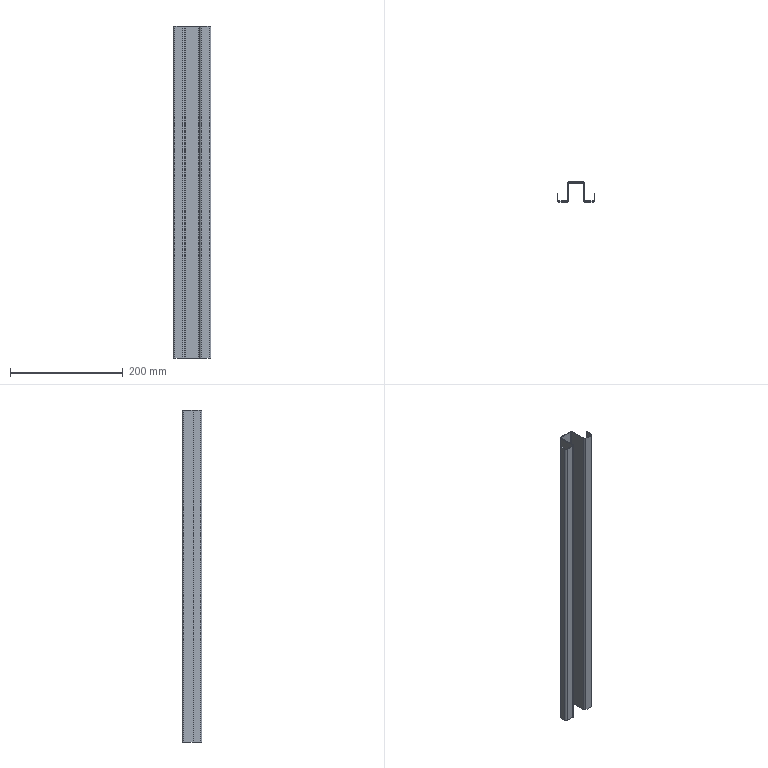Part | SolidWorks | features FlatPattern 1, SMBaseFlange 1, SheetMetal 1 | 1 solid | 54 faces | box 67 x 35 x 590 mm | volume 137357 mm3 | plane 42 | cylinder 12 | commonest cylinder face diameters 3 x6 6 x6
STEP:
#1=CARTESIAN_POINT('',(-17.662,-4.135,590.));
#2=VERTEX_POINT('',#1);
#3=CARTESIAN_POINT('',(-17.662,-5.635,590.));
#4=VERTEX_POINT('',#3);
#5=CARTESIAN_POINT('',(-17.662,-4.135,590.));
#6=DIRECTION('',(0.,-1.,0.));
#7=VECTOR('',#6,1000.);
#8=LINE('',#5,#7);
#9=EDGE_CURVE('',#2,#4,#8,.T.);
#10=ORIENTED_EDGE('',*,*,#9,.F.);
#11=CARTESIAN_POINT('',(-19.162,-2.635,590.));
#12=VERTEX_POINT('',#11);
#13=CARTESIAN_POINT('',(-17.662,-2.635,590.));
#14=DIRECTION('',(0.,0.,1.));
#15=DIRECTION('',(-1.,0.,0.));
#16=AXIS2_PLACEMENT_3D('',#13,#14,#15);
#17=CIRCLE('',#16,1.5);
#18=EDGE_CURVE('',#12,#2,#17,.T.);
#19=ORIENTED_EDGE('',*,*,#18,.F.);
#20=CARTESIAN_POINT('',(-20.662,-2.635,590.));
#21=VERTEX_POINT('',#20);
#22=CARTESIAN_POINT('',(-20.662,-2.635,590.));
#23=DIRECTION('',(1.,0.,0.));
#24=VECTOR('',#23,1000.);
#25=LINE('',#22,#24);
#26=EDGE_CURVE('',#21,#12,#25,.T.);
#27=ORIENTED_EDGE('',*,*,#26,.F.);
#28=CARTESIAN_POINT('',(-17.662,-2.635,590.));
#29=DIRECTION('',(0.,0.,1.));
#30=DIRECTION('',(1.,0.,0.));
#31=AXIS2_PLACEMENT_3D('',#28,#29,#30);
#32=CIRCLE('',#31,3.);
#33=EDGE_CURVE('',#21,#4,#32,.T.);
#34=ORIENTED_EDGE('',*,*,#33,.T.);
#35=EDGE_LOOP('',(#10,#19,#27,#34));
#36=FACE_OUTER_BOUND('',#35,.T.);
#37=CARTESIAN_POINT('',(-17.662,-4.135,590.));
#38=DIRECTION('',(0.,0.,1.));
#39=DIRECTION('',(1.,0.,0.));
#40=AXIS2_PLACEMENT_3D('',#37,#38,#39);
#41=PLANE('',#40);
#42=ADVANCED_FACE('',(#36),#41,.T.);
#43=CARTESIAN_POINT('',(-3.662,-4.135,590.));
#44=VERTEX_POINT('',#43);
#45=CARTESIAN_POINT('',(-19.162,-4.135,590.));
#46=DIRECTION('',(1.,0.,0.));
#47=VECTOR('',#46,1000.);
#48=LINE('',#45,#47);
#49=EDGE_CURVE('',#2,#44,#48,.T.);
#50=ORIENTED_EDGE('',*,*,#49,.F.);
#51=ORIENTED_EDGE('',*,*,#9,.T.);
#52=CARTESIAN_POINT('',(-3.662,-5.635,590.));
#53=VERTEX_POINT('',#52);
#54=CARTESIAN_POINT('',(-19.162,-5.635,590.));
#55=DIRECTION('',(1.,0.,0.));
#56=VECTOR('',#55,1000.);
#57=LINE('',#54,#56);
#58=EDGE_CURVE('',#4,#53,#57,.T.);
#59=ORIENTED_EDGE('',*,*,#58,.T.);
#60=CARTESIAN_POINT('',(-3.662,-5.635,590.));
#61=DIRECTION('',(0.,1.,0.));
#62=VECTOR('',#61,1000.);
#63=LINE('',#60,#62);
#64=EDGE_CURVE('',#53,#44,#63,.T.);
#65=ORIENTED_EDGE('',*,*,#64,.T.);
#66=EDGE_LOOP('',(#50,#51,#59,#65));
#67=FACE_OUTER_BOUND('',#66,.T.);
#68=CARTESIAN_POINT('',(-20.662,-2.635,590.));
#69=DIRECTION('',(0.,0.,1.));
#70=DIRECTION('',(1.,0.,0.));
#71=AXIS2_PLACEMENT_3D('',#68,#69,#70);
#72=PLANE('',#71);
#73=ADVANCED_FACE('',(#67),#72,.T.);
#74=CARTESIAN_POINT('',(-19.162,-2.635,0.));
#75=VERTEX_POINT('',#74);
#76=CARTESIAN_POINT('',(-20.662,-2.635,0.));
#77=VERTEX_POINT('',#76);
#78=CARTESIAN_POINT('',(-19.162,-2.635,0.));
#79=DIRECTION('',(-1.,0.,0.));
#80=VECTOR('',#79,1000.);
#81=LINE('',#78,#80);
#82=EDGE_CURVE('',#75,#77,#81,.T.);
#83=ORIENTED_EDGE('',*,*,#82,.F.);
#84=CARTESIAN_POINT('',(-17.662,-4.135,0.));
#85=VERTEX_POINT('',#84);
#86=CARTESIAN_POINT('',(-17.662,-2.635,0.));
#87=DIRECTION('',(0.,0.,1.));
#88=DIRECTION('',(-1.,0.,0.));
#89=AXIS2_PLACEMENT_3D('',#86,#87,#88);
#90=CIRCLE('',#89,1.5);
#91=EDGE_CURVE('',#75,#85,#90,.T.);
#92=ORIENTED_EDGE('',*,*,#91,.T.);
#93=CARTESIAN_POINT('',(-17.662,-5.635,0.));
#94=VERTEX_POINT('',#93);
#95=CARTESIAN_POINT('',(-17.662,-5.635,0.));
#96=DIRECTION('',(0.,1.,0.));
#97=VECTOR('',#96,1000.);
#98=LINE('',#95,#97);
#99=EDGE_CURVE('',#94,#85,#98,.T.);
#100=ORIENTED_EDGE('',*,*,#99,.F.);
#101=CARTESIAN_POINT('',(-17.662,-2.635,0.));
#102=DIRECTION('',(0.,0.,1.));
#103=DIRECTION('',(1.,0.,0.));
#104=AXIS2_PLACEMENT_3D('',#101,#102,#103);
#105=CIRCLE('',#104,3.);
#106=EDGE_CURVE('',#77,#94,#105,.T.);
#107=ORIENTED_EDGE('',*,*,#106,.F.);
#108=EDGE_LOOP('',(#83,#92,#100,#107));
#109=FACE_OUTER_BOUND('',#108,.T.);
#110=CARTESIAN_POINT('',(-19.162,-2.635,0.));
#111=DIRECTION('',(0.,0.,-1.));
#112=DIRECTION('',(-1.,0.,0.));
#113=AXIS2_PLACEMENT_3D('',#110,#111,#112);
#114=PLANE('',#113);
#115=ADVANCED_FACE('',(#109),#114,.T.);
#116=CARTESIAN_POINT('',(-19.162,9.365,0.));
#117=VERTEX_POINT('',#116);
#118=CARTESIAN_POINT('',(-19.162,9.365,0.));
#119=DIRECTION('',(0.,-1.,0.));
#120=VECTOR('',#119,1000.);
#121=LINE('',#118,#120);
#122=EDGE_CURVE('',#117,#75,#121,.T.);
#123=ORIENTED_EDGE('',*,*,#122,.T.);
#124=ORIENTED_EDGE('',*,*,#82,.T.);
#125=CARTESIAN_POINT('',(-20.662,9.365,0.));
#126=VERTEX_POINT('',#125);
#127=CARTESIAN_POINT('',(-20.662,9.365,0.));
#128=DIRECTION('',(0.,-1.,0.));
#129=VECTOR('',#128,1000.);
#130=LINE('',#127,#129);
#131=EDGE_CURVE('',#126,#77,#130,.T.);
#132=ORIENTED_EDGE('',*,*,#131,.F.);
#133=CARTESIAN_POINT('',(-20.662,9.365,0.));
#134=DIRECTION('',(1.,0.,0.));
#135=VECTOR('',#134,1000.);
#136=LINE('',#133,#135);
#137=EDGE_CURVE('',#126,#117,#136,.T.);
#138=ORIENTED_EDGE('',*,*,#137,.T.);
#139=EDGE_LOOP('',(#123,#124,#132,#138));
#140=FACE_OUTER_BOUND('',#139,.T.);
#141=CARTESIAN_POINT('',(-17.662,-5.635,0.));
#142=DIRECTION('',(0.,0.,-1.));
#143=DIRECTION('',(-1.,0.,0.));
#144=AXIS2_PLACEMENT_3D('',#141,#142,#143);
#145=PLANE('',#144);
#146=ADVANCED_FACE('',(#140),#145,.T.);
#147=CARTESIAN_POINT('',(-2.162,-2.635,590.));
#148=VERTEX_POINT('',#147);
#149=CARTESIAN_POINT('',(-0.6616,-2.635,590.));
#150=VERTEX_POINT('',#149);
#151=CARTESIAN_POINT('',(-2.162,-2.635,590.));
#152=DIRECTION('',(1.,0.,0.));
#153=VECTOR('',#152,1000.);
#154=LINE('',#151,#153);
#155=EDGE_CURVE('',#148,#150,#154,.T.);
#156=ORIENTED_EDGE('',*,*,#155,.F.);
#157=CARTESIAN_POINT('',(-3.662,-2.635,590.));
#158=DIRECTION('',(0.,0.,1.));
#159=DIRECTION('',(-1.,0.,0.));
#160=AXIS2_PLACEMENT_3D('',#157,#158,#159);
#161=CIRCLE('',#160,1.5);
#162=EDGE_CURVE('',#44,#148,#161,.T.);
#163=ORIENTED_EDGE('',*,*,#162,.F.);
#164=ORIENTED_EDGE('',*,*,#64,.F.);
#165=CARTESIAN_POINT('',(-3.662,-2.635,590.));
#166=DIRECTION('',(0.,0.,1.));
#167=DIRECTION('',(1.,0.,0.));
#168=AXIS2_PLACEMENT_3D('',#165,#166,#167);
#169=CIRCLE('',#168,3.);
#170=EDGE_CURVE('',#53,#150,#169,.T.);
#171=ORIENTED_EDGE('',*,*,#170,.T.);
#172=EDGE_LOOP('',(#156,#163,#164,#171));
#173=FACE_OUTER_BOUND('',#172,.T.);
#174=CARTESIAN_POINT('',(-2.162,-2.635,590.));
#175=DIRECTION('',(0.,0.,1.));
#176=DIRECTION('',(1.,0.,0.));
#177=AXIS2_PLACEMENT_3D('',#174,#175,#176);
#178=PLANE('',#177);
#179=ADVANCED_FACE('',(#173),#178,.T.);
#180=CARTESIAN_POINT('',(-2.162,26.365,590.));
#181=VERTEX_POINT('',#180);
#182=CARTESIAN_POINT('',(-2.162,-4.135,590.));
#183=DIRECTION('',(0.,1.,0.));
#184=VECTOR('',#183,1000.);
#185=LINE('',#182,#184);
#186=EDGE_CURVE('',#148,#181,#185,.T.);
#187=ORIENTED_EDGE('',*,*,#186,.F.);
#188=ORIENTED_EDGE('',*,*,#155,.T.);
#189=CARTESIAN_POINT('',(-0.6616,26.365,590.));
#190=VERTEX_POINT('',#189);
#191=CARTESIAN_POINT('',(-0.6616,-4.135,590.));
#192=DIRECTION('',(0.,1.,0.));
#193=VECTOR('',#192,1000.);
#194=LINE('',#191,#193);
#195=EDGE_CURVE('',#150,#190,#194,.T.);
#196=ORIENTED_EDGE('',*,*,#195,.T.);
#197=CARTESIAN_POINT('',(-0.6616,26.365,590.));
#198=DIRECTION('',(-1.,0.,0.));
#199=VECTOR('',#198,1000.);
#200=LINE('',#197,#199);
#201=EDGE_CURVE('',#190,#181,#200,.T.);
#202=ORIENTED_EDGE('',*,*,#201,.T.);
#203=EDGE_LOOP('',(#187,#188,#196,#202));
#204=FACE_OUTER_BOUND('',#203,.T.);
#205=CARTESIAN_POINT('',(-3.662,-5.635,590.));
#206=DIRECTION('',(0.,0.,1.));
#207=DIRECTION('',(1.,0.,0.));
#208=AXIS2_PLACEMENT_3D('',#205,#206,#207);
#209=PLANE('',#208);
#210=ADVANCED_FACE('',(#204),#209,.T.);
#211=CARTESIAN_POINT('',(-3.662,-4.135,0.));
#212=VERTEX_POINT('',#211);
#213=CARTESIAN_POINT('',(-3.662,-5.635,0.));
#214=VERTEX_POINT('',#213);
#215=CARTESIAN_POINT('',(-3.662,-4.135,0.));
#216=DIRECTION('',(0.,-1.,0.));
#217=VECTOR('',#216,1000.);
#218=LINE('',#215,#217);
#219=EDGE_CURVE('',#212,#214,#218,.T.);
#220=ORIENTED_EDGE('',*,*,#219,.F.);
#221=CARTESIAN_POINT('',(-2.162,-2.635,0.));
#222=VERTEX_POINT('',#221);
#223=CARTESIAN_POINT('',(-3.662,-2.635,0.));
#224=DIRECTION('',(0.,0.,1.));
#225=DIRECTION('',(-1.,0.,0.));
#226=AXIS2_PLACEMENT_3D('',#223,#224,#225);
#227=CIRCLE('',#226,1.5);
#228=EDGE_CURVE('',#212,#222,#227,.T.);
#229=ORIENTED_EDGE('',*,*,#228,.T.);
#230=CARTESIAN_POINT('',(-0.6616,-2.635,0.));
#231=VERTEX_POINT('',#230);
#232=CARTESIAN_POINT('',(-0.6616,-2.635,0.));
#233=DIRECTION('',(-1.,0.,0.));
#234=VECTOR('',#233,1000.);
#235=LINE('',#232,#234);
#236=EDGE_CURVE('',#231,#222,#235,.T.);
#237=ORIENTED_EDGE('',*,*,#236,.F.);
#238=CARTESIAN_POINT('',(-3.662,-2.635,0.));
#239=DIRECTION('',(0.,0.,1.));
#240=DIRECTION('',(1.,0.,0.));
#241=AXIS2_PLACEMENT_3D('',#238,#239,#240);
#242=CIRCLE('',#241,3.);
#243=EDGE_CURVE('',#214,#231,#242,.T.);
#244=ORIENTED_EDGE('',*,*,#243,.F.);
#245=EDGE_LOOP('',(#220,#229,#237,#244));
#246=FACE_OUTER_BOUND('',#245,.T.);
#247=CARTESIAN_POINT('',(-3.662,-4.135,0.));
#248=DIRECTION('',(0.,0.,-1.));
#249=DIRECTION('',(-1.,0.,0.));
#250=AXIS2_PLACEMENT_3D('',#247,#248,#249);
#251=PLANE('',#250);
#252=ADVANCED_FACE('',(#246),#251,.T.);
#253=CARTESIAN_POINT('',(-19.162,-4.135,0.));
#254=DIRECTION('',(1.,0.,0.));
#255=VECTOR('',#254,1000.);
#256=LINE('',#253,#255);
#257=EDGE_CURVE('',#85,#212,#256,.T.);
#258=ORIENTED_EDGE('',*,*,#257,.T.);
#259=ORIENTED_EDGE('',*,*,#219,.T.);
#260=CARTESIAN_POINT('',(-19.162,-5.635,0.));
#261=DIRECTION('',(1.,0.,0.));
#262=VECTOR('',#261,1000.);
#263=LINE('',#260,#262);
#264=EDGE_CURVE('',#94,#214,#263,.T.);
#265=ORIENTED_EDGE('',*,*,#264,.F.);
#266=ORIENTED_EDGE('',*,*,#99,.T.);
#267=EDGE_LOOP('',(#258,#259,#265,#266));
#268=FACE_OUTER_BOUND('',#267,.T.);
#269=CARTESIAN_POINT('',(-0.6616,-2.635,0.));
#270=DIRECTION('',(0.,0.,-1.));
#271=DIRECTION('',(-1.,0.,0.));
#272=AXIS2_PLACEMENT_3D('',#269,#270,#271);
#273=PLANE('',#272);
#274=ADVANCED_FACE('',(#268),#273,.T.);
#275=CARTESIAN_POINT('',(0.8384,29.365,590.));
#276=VERTEX_POINT('',#275);
#277=CARTESIAN_POINT('',(0.8384,27.865,590.));
#278=VERTEX_POINT('',#277);
#279=CARTESIAN_POINT('',(0.8384,29.365,590.));
#280=DIRECTION('',(0.,-1.,0.));
#281=VECTOR('',#280,1000.);
#282=LINE('',#279,#281);
#283=EDGE_CURVE('',#276,#278,#282,.T.);
#284=ORIENTED_EDGE('',*,*,#283,.F.);
#285=CARTESIAN_POINT('',(0.8384,26.365,590.));
#286=DIRECTION('',(0.,0.,-1.));
#287=DIRECTION('',(1.,0.,0.));
#288=AXIS2_PLACEMENT_3D('',#285,#286,#287);
#289=CIRCLE('',#288,3.);
#290=EDGE_CURVE('',#181,#276,#289,.T.);
#291=ORIENTED_EDGE('',*,*,#290,.F.);
#292=ORIENTED_EDGE('',*,*,#201,.F.);
#293=CARTESIAN_POINT('',(0.8384,26.365,590.));
#294=DIRECTION('',(0.,0.,-1.));
#295=DIRECTION('',(1.,0.,0.));
#296=AXIS2_PLACEMENT_3D('',#293,#294,#295);
#297=CIRCLE('',#296,1.5);
#298=EDGE_CURVE('',#190,#278,#297,.T.);
#299=ORIENTED_EDGE('',*,*,#298,.T.);
#300=EDGE_LOOP('',(#284,#291,#292,#299));
#301=FACE_OUTER_BOUND('',#300,.T.);
#302=CARTESIAN_POINT('',(0.8384,29.365,590.));
#303=DIRECTION('',(0.,0.,1.));
#304=DIRECTION('',(1.,0.,0.));
#305=AXIS2_PLACEMENT_3D('',#302,#303,#304);
#306=PLANE('',#305);
#307=ADVANCED_FACE('',(#301),#306,.T.);
#308=CARTESIAN_POINT('',(24.838,29.365,590.));
#309=VERTEX_POINT('',#308);
#310=CARTESIAN_POINT('',(-2.162,29.365,590.));
#311=DIRECTION('',(1.,0.,0.));
#312=VECTOR('',#311,1000.);
#313=LINE('',#310,#312);
#314=EDGE_CURVE('',#276,#309,#313,.T.);
#315=ORIENTED_EDGE('',*,*,#314,.F.);
#316=ORIENTED_EDGE('',*,*,#283,.T.);
#317=CARTESIAN_POINT('',(24.838,27.865,590.));
#318=VERTEX_POINT('',#317);
#319=CARTESIAN_POINT('',(-2.162,27.865,590.));
#320=DIRECTION('',(1.,0.,0.));
#321=VECTOR('',#320,1000.);
#322=LINE('',#319,#321);
#323=EDGE_CURVE('',#278,#318,#322,.T.);
#324=ORIENTED_EDGE('',*,*,#323,.T.);
#325=CARTESIAN_POINT('',(24.838,27.865,590.));
#326=DIRECTION('',(0.,1.,0.));
#327=VECTOR('',#326,1000.);
#328=LINE('',#325,#327);
#329=EDGE_CURVE('',#318,#309,#328,.T.);
#330=ORIENTED_EDGE('',*,*,#329,.T.);
#331=EDGE_LOOP('',(#315,#316,#324,#330));
#332=FACE_OUTER_BOUND('',#331,.T.);
#333=CARTESIAN_POINT('',(-0.6616,26.365,590.));
#334=DIRECTION('',(0.,0.,1.));
#335=DIRECTION('',(1.,0.,0.));
#336=AXIS2_PLACEMENT_3D('',#333,#334,#335);
#337=PLANE('',#336);
#338=ADVANCED_FACE('',(#332),#337,.T.);
#339=CARTESIAN_POINT('',(-2.162,26.365,0.));
#340=VERTEX_POINT('',#339);
#341=CARTESIAN_POINT('',(-0.6616,26.365,0.));
#342=VERTEX_POINT('',#341);
#343=CARTESIAN_POINT('',(-2.162,26.365,0.));
#344=DIRECTION('',(1.,0.,0.));
#345=VECTOR('',#344,1000.);
#346=LINE('',#343,#345);
#347=EDGE_CURVE('',#340,#342,#346,.T.);
#348=ORIENTED_EDGE('',*,*,#347,.F.);
#349=CARTESIAN_POINT('',(0.8384,29.365,0.));
#350=VERTEX_POINT('',#349);
#351=CARTESIAN_POINT('',(0.8384,26.365,0.));
#352=DIRECTION('',(0.,0.,-1.));
#353=DIRECTION('',(1.,0.,0.));
#354=AXIS2_PLACEMENT_3D('',#351,#352,#353);
#355=CIRCLE('',#354,3.);
#356=EDGE_CURVE('',#340,#350,#355,.T.);
#357=ORIENTED_EDGE('',*,*,#356,.T.);
#358=CARTESIAN_POINT('',(0.8384,27.865,0.));
#359=VERTEX_POINT('',#358);
#360=CARTESIAN_POINT('',(0.8384,27.865,0.));
#361=DIRECTION('',(0.,1.,0.));
#362=VECTOR('',#361,1000.);
#363=LINE('',#360,#362);
#364=EDGE_CURVE('',#359,#350,#363,.T.);
#365=ORIENTED_EDGE('',*,*,#364,.F.);
#366=CARTESIAN_POINT('',(0.8384,26.365,0.));
#367=DIRECTION('',(0.,0.,-1.));
#368=DIRECTION('',(1.,0.,0.));
#369=AXIS2_PLACEMENT_3D('',#366,#367,#368);
#370=CIRCLE('',#369,1.5);
#371=EDGE_CURVE('',#342,#359,#370,.T.);
#372=ORIENTED_EDGE('',*,*,#371,.F.);
#373=EDGE_LOOP('',(#348,#357,#365,#372));
#374=FACE_OUTER_BOUND('',#373,.T.);
#375=CARTESIAN_POINT('',(-2.162,26.365,0.));
#376=DIRECTION('',(0.,0.,-1.));
#377=DIRECTION('',(-1.,0.,0.));
#378=AXIS2_PLACEMENT_3D('',#375,#376,#377);
#379=PLANE('',#378);
#380=ADVANCED_FACE('',(#374),#379,.T.);
#381=CARTESIAN_POINT('',(-2.162,-4.135,0.));
#382=DIRECTION('',(0.,1.,0.));
#383=VECTOR('',#382,1000.);
#384=LINE('',#381,#383);
#385=EDGE_CURVE('',#222,#340,#384,.T.);
#386=ORIENTED_EDGE('',*,*,#385,.T.);
#387=ORIENTED_EDGE('',*,*,#347,.T.);
#388=CARTESIAN_POINT('',(-0.6616,-4.135,0.));
#389=DIRECTION('',(0.,1.,0.));
#390=VECTOR('',#389,1000.);
#391=LINE('',#388,#390);
#392=EDGE_CURVE('',#231,#342,#391,.T.);
#393=ORIENTED_EDGE('',*,*,#392,.F.);
#394=ORIENTED_EDGE('',*,*,#236,.T.);
#395=EDGE_LOOP('',(#386,#387,#393,#394));
#396=FACE_OUTER_BOUND('',#395,.T.);
#397=CARTESIAN_POINT('',(0.8384,27.865,0.));
#398=DIRECTION('',(0.,0.,-1.));
#399=DIRECTION('',(-1.,0.,0.));
#400=AXIS2_PLACEMENT_3D('',#397,#398,#399);
#401=PLANE('',#400);
#402=ADVANCED_FACE('',(#396),#401,.T.);
#403=CARTESIAN_POINT('',(27.838,26.365,590.));
#404=VERTEX_POINT('',#403);
#405=CARTESIAN_POINT('',(26.338,26.365,590.));
#406=VERTEX_POINT('',#405);
#407=CARTESIAN_POINT('',(27.838,26.365,590.));
#408=DIRECTION('',(-1.,0.,0.));
#409=VECTOR('',#408,1000.);
#410=LINE('',#407,#409);
#411=EDGE_CURVE('',#404,#406,#410,.T.);
#412=ORIENTED_EDGE('',*,*,#411,.F.);
#413=CARTESIAN_POINT('',(24.838,26.365,590.));
#414=DIRECTION('',(0.,0.,-1.));
#415=DIRECTION('',(1.,0.,0.));
#416=AXIS2_PLACEMENT_3D('',#413,#414,#415);
#417=CIRCLE('',#416,3.);
#418=EDGE_CURVE('',#309,#404,#417,.T.);
#419=ORIENTED_EDGE('',*,*,#418,.F.);
#420=ORIENTED_EDGE('',*,*,#329,.F.);
#421=CARTESIAN_POINT('',(24.838,26.365,590.));
#422=DIRECTION('',(0.,0.,-1.));
#423=DIRECTION('',(1.,0.,0.));
#424=AXIS2_PLACEMENT_3D('',#421,#422,#423);
#425=CIRCLE('',#424,1.5);
#426=EDGE_CURVE('',#318,#406,#425,.T.);
#427=ORIENTED_EDGE('',*,*,#426,.T.);
#428=EDGE_LOOP('',(#412,#419,#420,#427));
#429=FACE_OUTER_BOUND('',#428,.T.);
#430=CARTESIAN_POINT('',(27.838,26.365,590.));
#431=DIRECTION('',(0.,0.,1.));
#432=DIRECTION('',(1.,0.,0.));
#433=AXIS2_PLACEMENT_3D('',#430,#431,#432);
#434=PLANE('',#433);
#435=ADVANCED_FACE('',(#429),#434,.T.);
#436=CARTESIAN_POINT('',(27.838,-2.635,590.));
#437=VERTEX_POINT('',#436);
#438=CARTESIAN_POINT('',(27.838,29.365,590.));
#439=DIRECTION('',(0.,-1.,0.));
#440=VECTOR('',#439,1000.);
#441=LINE('',#438,#440);
#442=EDGE_CURVE('',#404,#437,#441,.T.);
#443=ORIENTED_EDGE('',*,*,#442,.F.);
#444=ORIENTED_EDGE('',*,*,#411,.T.);
#445=CARTESIAN_POINT('',(26.338,-2.635,590.));
#446=VERTEX_POINT('',#445);
#447=CARTESIAN_POINT('',(26.338,29.365,590.));
#448=DIRECTION('',(0.,-1.,0.));
#449=VECTOR('',#448,1000.);
#450=LINE('',#447,#449);
#451=EDGE_CURVE('',#406,#446,#450,.T.);
#452=ORIENTED_EDGE('',*,*,#451,.T.);
#453=CARTESIAN_POINT('',(26.338,-2.635,590.));
#454=DIRECTION('',(1.,0.,0.));
#455=VECTOR('',#454,1000.);
#456=LINE('',#453,#455);
#457=EDGE_CURVE('',#446,#437,#456,.T.);
#458=ORIENTED_EDGE('',*,*,#457,.T.);
#459=EDGE_LOOP('',(#443,#444,#452,#458));
#460=FACE_OUTER_BOUND('',#459,.T.);
#461=CARTESIAN_POINT('',(24.838,27.865,590.));
#462=DIRECTION('',(0.,0.,1.));
#463=DIRECTION('',(1.,0.,0.));
#464=AXIS2_PLACEMENT_3D('',#461,#462,#463);
#465=PLANE('',#464);
#466=ADVANCED_FACE('',(#460),#465,.T.);
#467=CARTESIAN_POINT('',(24.838,29.365,0.));
#468=VERTEX_POINT('',#467);
#469=CARTESIAN_POINT('',(24.838,27.865,0.));
#470=VERTEX_POINT('',#469);
#471=CARTESIAN_POINT('',(24.838,29.365,0.));
#472=DIRECTION('',(0.,-1.,0.));
#473=VECTOR('',#472,1000.);
#474=LINE('',#471,#473);
#475=EDGE_CURVE('',#468,#470,#474,.T.);
#476=ORIENTED_EDGE('',*,*,#475,.F.);
#477=CARTESIAN_POINT('',(27.838,26.365,0.));
#478=VERTEX_POINT('',#477);
#479=CARTESIAN_POINT('',(24.838,26.365,0.));
#480=DIRECTION('',(0.,0.,-1.));
#481=DIRECTION('',(1.,0.,0.));
#482=AXIS2_PLACEMENT_3D('',#479,#480,#481);
#483=CIRCLE('',#482,3.);
#484=EDGE_CURVE('',#468,#478,#483,.T.);
#485=ORIENTED_EDGE('',*,*,#484,.T.);
#486=CARTESIAN_POINT('',(26.338,26.365,0.));
#487=VERTEX_POINT('',#486);
#488=CARTESIAN_POINT('',(26.338,26.365,0.));
#489=DIRECTION('',(1.,0.,0.));
#490=VECTOR('',#489,1000.);
#491=LINE('',#488,#490);
#492=EDGE_CURVE('',#487,#478,#491,.T.);
#493=ORIENTED_EDGE('',*,*,#492,.F.);
#494=CARTESIAN_POINT('',(24.838,26.365,0.));
#495=DIRECTION('',(0.,0.,-1.));
#496=DIRECTION('',(1.,0.,0.));
#497=AXIS2_PLACEMENT_3D('',#494,#495,#496);
#498=CIRCLE('',#497,1.5);
#499=EDGE_CURVE('',#470,#487,#498,.T.);
#500=ORIENTED_EDGE('',*,*,#499,.F.);
#501=EDGE_LOOP('',(#476,#485,#493,#500));
#502=FACE_OUTER_BOUND('',#501,.T.);
#503=CARTESIAN_POINT('',(24.838,29.365,0.));
#504=DIRECTION('',(0.,0.,-1.));
#505=DIRECTION('',(-1.,0.,0.));
#506=AXIS2_PLACEMENT_3D('',#503,#504,#505);
#507=PLANE('',#506);
#508=ADVANCED_FACE('',(#502),#507,.T.);
#509=CARTESIAN_POINT('',(-2.162,29.365,0.));
#510=DIRECTION('',(1.,0.,0.));
#511=VECTOR('',#510,1000.);
#512=LINE('',#509,#511);
#513=EDGE_CURVE('',#350,#468,#512,.T.);
#514=ORIENTED_EDGE('',*,*,#513,.T.);
#515=ORIENTED_EDGE('',*,*,#475,.T.);
#516=CARTESIAN_POINT('',(-2.162,27.865,0.));
#517=DIRECTION('',(1.,0.,0.));
#518=VECTOR('',#517,1000.);
#519=LINE('',#516,#518);
#520=EDGE_CURVE('',#359,#470,#519,.T.);
#521=ORIENTED_EDGE('',*,*,#520,.F.);
#522=ORIENTED_EDGE('',*,*,#364,.T.);
#523=EDGE_LOOP('',(#514,#515,#521,#522));
#524=FACE_OUTER_BOUND('',#523,.T.);
#525=CARTESIAN_POINT('',(26.338,26.365,0.));
#526=DIRECTION('',(0.,0.,-1.));
#527=DIRECTION('',(-1.,0.,0.));
#528=AXIS2_PLACEMENT_3D('',#525,#526,#527);
#529=PLANE('',#528);
#530=ADVANCED_FACE('',(#524),#529,.T.);
#531=CARTESIAN_POINT('',(29.338,-4.135,590.));
#532=VERTEX_POINT('',#531);
#533=CARTESIAN_POINT('',(29.338,-5.635,590.));
#534=VERTEX_POINT('',#533);
#535=CARTESIAN_POINT('',(29.338,-4.135,590.));
#536=DIRECTION('',(0.,-1.,0.));
#537=VECTOR('',#536,1000.);
#538=LINE('',#535,#537);
#539=EDGE_CURVE('',#532,#534,#538,.T.);
#540=ORIENTED_EDGE('',*,*,#539,.F.);
#541=CARTESIAN_POINT('',(29.338,-2.635,590.));
#542=DIRECTION('',(0.,0.,1.));
#543=DIRECTION('',(-1.,0.,0.));
#544=AXIS2_PLACEMENT_3D('',#541,#542,#543);
#545=CIRCLE('',#544,1.5);
#546=EDGE_CURVE('',#437,#532,#545,.T.);
#547=ORIENTED_EDGE('',*,*,#546,.F.);
#548=ORIENTED_EDGE('',*,*,#457,.F.);
#549=CARTESIAN_POINT('',(29.338,-2.635,590.));
#550=DIRECTION('',(0.,0.,1.));
#551=DIRECTION('',(1.,0.,0.));
#552=AXIS2_PLACEMENT_3D('',#549,#550,#551);
#553=CIRCLE('',#552,3.);
#554=EDGE_CURVE('',#446,#534,#553,.T.);
#555=ORIENTED_EDGE('',*,*,#554,.T.);
#556=EDGE_LOOP('',(#540,#547,#548,#555));
#557=FACE_OUTER_BOUND('',#556,.T.);
#558=CARTESIAN_POINT('',(29.338,-4.135,590.));
#559=DIRECTION('',(0.,0.,1.));
#560=DIRECTION('',(1.,0.,0.));
#561=AXIS2_PLACEMENT_3D('',#558,#559,#560);
#562=PLANE('',#561);
#563=ADVANCED_FACE('',(#557),#562,.T.);
#564=CARTESIAN_POINT('',(43.338,-4.135,590.));
#565=VERTEX_POINT('',#564);
#566=CARTESIAN_POINT('',(27.838,-4.135,590.));
#567=DIRECTION('',(1.,0.,0.));
#568=VECTOR('',#567,1000.);
#569=LINE('',#566,#568);
#570=EDGE_CURVE('',#532,#565,#569,.T.);
#571=ORIENTED_EDGE('',*,*,#570,.F.);
#572=ORIENTED_EDGE('',*,*,#539,.T.);
#573=CARTESIAN_POINT('',(43.338,-5.635,590.));
#574=VERTEX_POINT('',#573);
#575=CARTESIAN_POINT('',(27.838,-5.635,590.));
#576=DIRECTION('',(1.,0.,0.));
#577=VECTOR('',#576,1000.);
#578=LINE('',#575,#577);
#579=EDGE_CURVE('',#534,#574,#578,.T.);
#580=ORIENTED_EDGE('',*,*,#579,.T.);
#581=CARTESIAN_POINT('',(43.338,-5.635,590.));
#582=DIRECTION('',(0.,1.,0.));
#583=VECTOR('',#582,1000.);
#584=LINE('',#581,#583);
#585=EDGE_CURVE('',#574,#565,#584,.T.);
#586=ORIENTED_EDGE('',*,*,#585,.T.);
#587=EDGE_LOOP('',(#571,#572,#580,#586));
#588=FACE_OUTER_BOUND('',#587,.T.);
#589=CARTESIAN_POINT('',(26.338,-2.635,590.));
#590=DIRECTION('',(0.,0.,1.));
#591=DIRECTION('',(1.,0.,0.));
#592=AXIS2_PLACEMENT_3D('',#589,#590,#591);
#593=PLANE('',#592);
#594=ADVANCED_FACE('',(#588),#593,.T.);
#595=CARTESIAN_POINT('',(27.838,-2.635,0.));
#596=VERTEX_POINT('',#595);
#597=CARTESIAN_POINT('',(26.338,-2.635,0.));
#598=VERTEX_POINT('',#597);
#599=CARTESIAN_POINT('',(27.838,-2.635,0.));
#600=DIRECTION('',(-1.,0.,0.));
#601=VECTOR('',#600,1000.);
#602=LINE('',#599,#601);
#603=EDGE_CURVE('',#596,#598,#602,.T.);
#604=ORIENTED_EDGE('',*,*,#603,.F.);
#605=CARTESIAN_POINT('',(29.338,-4.135,0.));
#606=VERTEX_POINT('',#605);
#607=CARTESIAN_POINT('',(29.338,-2.635,0.));
#608=DIRECTION('',(0.,0.,1.));
#609=DIRECTION('',(-1.,0.,0.));
#610=AXIS2_PLACEMENT_3D('',#607,#608,#609);
#611=CIRCLE('',#610,1.5);
#612=EDGE_CURVE('',#596,#606,#611,.T.);
#613=ORIENTED_EDGE('',*,*,#612,.T.);
#614=CARTESIAN_POINT('',(29.338,-5.635,0.));
#615=VERTEX_POINT('',#614);
#616=CARTESIAN_POINT('',(29.338,-5.635,0.));
#617=DIRECTION('',(0.,1.,0.));
#618=VECTOR('',#617,1000.);
#619=LINE('',#616,#618);
#620=EDGE_CURVE('',#615,#606,#619,.T.);
#621=ORIENTED_EDGE('',*,*,#620,.F.);
#622=CARTESIAN_POINT('',(29.338,-2.635,0.));
#623=DIRECTION('',(0.,0.,1.));
#624=DIRECTION('',(1.,0.,0.));
#625=AXIS2_PLACEMENT_3D('',#622,#623,#624);
#626=CIRCLE('',#625,3.);
#627=EDGE_CURVE('',#598,#615,#626,.T.);
#628=ORIENTED_EDGE('',*,*,#627,.F.);
#629=EDGE_LOOP('',(#604,#613,#621,#628));
#630=FACE_OUTER_BOUND('',#629,.T.);
#631=CARTESIAN_POINT('',(27.838,-2.635,0.));
#632=DIRECTION('',(0.,0.,-1.));
#633=DIRECTION('',(-1.,0.,0.));
#634=AXIS2_PLACEMENT_3D('',#631,#632,#633);
#635=PLANE('',#634);
#636=ADVANCED_FACE('',(#630),#635,.T.);
#637=CARTESIAN_POINT('',(27.838,29.365,0.));
#638=DIRECTION('',(0.,-1.,0.));
#639=VECTOR('',#638,1000.);
#640=LINE('',#637,#639);
#641=EDGE_CURVE('',#478,#596,#640,.T.);
#642=ORIENTED_EDGE('',*,*,#641,.T.);
#643=ORIENTED_EDGE('',*,*,#603,.T.);
#644=CARTESIAN_POINT('',(26.338,29.365,0.));
#645=DIRECTION('',(0.,-1.,0.));
#646=VECTOR('',#645,1000.);
#647=LINE('',#644,#646);
#648=EDGE_CURVE('',#487,#598,#647,.T.);
#649=ORIENTED_EDGE('',*,*,#648,.F.);
#650=ORIENTED_EDGE('',*,*,#492,.T.);
#651=EDGE_LOOP('',(#642,#643,#649,#650));
#652=FACE_OUTER_BOUND('',#651,.T.);
#653=CARTESIAN_POINT('',(29.338,-5.635,0.));
#654=DIRECTION('',(0.,0.,-1.));
#655=DIRECTION('',(-1.,0.,0.));
#656=AXIS2_PLACEMENT_3D('',#653,#654,#655);
#657=PLANE('',#656);
#658=ADVANCED_FACE('',(#652),#657,.T.);
#659=CARTESIAN_POINT('',(44.838,-2.635,590.));
#660=VERTEX_POINT('',#659);
#661=CARTESIAN_POINT('',(46.338,-2.635,590.));
#662=VERTEX_POINT('',#661);
#663=CARTESIAN_POINT('',(44.838,-2.635,590.));
#664=DIRECTION('',(1.,0.,0.));
#665=VECTOR('',#664,1000.);
#666=LINE('',#663,#665);
#667=EDGE_CURVE('',#660,#662,#666,.T.);
#668=ORIENTED_EDGE('',*,*,#667,.F.);
#669=CARTESIAN_POINT('',(43.338,-2.635,590.));
#670=DIRECTION('',(0.,0.,1.));
#671=DIRECTION('',(-1.,0.,0.));
#672=AXIS2_PLACEMENT_3D('',#669,#670,#671);
#673=CIRCLE('',#672,1.5);
#674=EDGE_CURVE('',#565,#660,#673,.T.);
#675=ORIENTED_EDGE('',*,*,#674,.F.);
#676=ORIENTED_EDGE('',*,*,#585,.F.);
#677=CARTESIAN_POINT('',(43.338,-2.635,590.));
#678=DIRECTION('',(0.,0.,1.));
#679=DIRECTION('',(1.,0.,0.));
#680=AXIS2_PLACEMENT_3D('',#677,#678,#679);
#681=CIRCLE('',#680,3.);
#682=EDGE_CURVE('',#574,#662,#681,.T.);
#683=ORIENTED_EDGE('',*,*,#682,.T.);
#684=EDGE_LOOP('',(#668,#675,#676,#683));
#685=FACE_OUTER_BOUND('',#684,.T.);
#686=CARTESIAN_POINT('',(44.838,-2.635,590.));
#687=DIRECTION('',(0.,0.,1.));
#688=DIRECTION('',(1.,0.,0.));
#689=AXIS2_PLACEMENT_3D('',#686,#687,#688);
#690=PLANE('',#689);
#691=ADVANCED_FACE('',(#685),#690,.T.);
#692=CARTESIAN_POINT('',(44.838,9.365,590.));
#693=VERTEX_POINT('',#692);
#694=CARTESIAN_POINT('',(44.838,-4.135,590.));
#695=DIRECTION('',(0.,1.,0.));
#696=VECTOR('',#695,1000.);
#697=LINE('',#694,#696);
#698=EDGE_CURVE('',#660,#693,#697,.T.);
#699=ORIENTED_EDGE('',*,*,#698,.F.);
#700=ORIENTED_EDGE('',*,*,#667,.T.);
#701=CARTESIAN_POINT('',(46.338,9.365,590.));
#702=VERTEX_POINT('',#701);
#703=CARTESIAN_POINT('',(46.338,-4.135,590.));
#704=DIRECTION('',(0.,1.,0.));
#705=VECTOR('',#704,1000.);
#706=LINE('',#703,#705);
#707=EDGE_CURVE('',#662,#702,#706,.T.);
#708=ORIENTED_EDGE('',*,*,#707,.T.);
#709=CARTESIAN_POINT('',(44.838,9.365,590.));
#710=DIRECTION('',(1.,0.,0.));
#711=VECTOR('',#710,1000.);
#712=LINE('',#709,#711);
#713=EDGE_CURVE('',#693,#702,#712,.T.);
#714=ORIENTED_EDGE('',*,*,#713,.F.);
#715=EDGE_LOOP('',(#699,#700,#708,#714));
#716=FACE_OUTER_BOUND('',#715,.T.);
#717=CARTESIAN_POINT('',(43.338,-5.635,590.));
#718=DIRECTION('',(0.,0.,1.));
#719=DIRECTION('',(1.,0.,0.));
#720=AXIS2_PLACEMENT_3D('',#717,#718,#719);
#721=PLANE('',#720);
#722=ADVANCED_FACE('',(#716),#721,.T.);
#723=CARTESIAN_POINT('',(43.338,-4.135,0.));
#724=VERTEX_POINT('',#723);
#725=CARTESIAN_POINT('',(43.338,-5.635,0.));
#726=VERTEX_POINT('',#725);
#727=CARTESIAN_POINT('',(43.338,-4.135,0.));
#728=DIRECTION('',(0.,-1.,0.));
#729=VECTOR('',#728,1000.);
#730=LINE('',#727,#729);
#731=EDGE_CURVE('',#724,#726,#730,.T.);
#732=ORIENTED_EDGE('',*,*,#731,.F.);
#733=CARTESIAN_POINT('',(44.838,-2.635,0.));
#734=VERTEX_POINT('',#733);
#735=CARTESIAN_POINT('',(43.338,-2.635,0.));
#736=DIRECTION('',(0.,0.,1.));
#737=DIRECTION('',(-1.,0.,0.));
#738=AXIS2_PLACEMENT_3D('',#735,#736,#737);
#739=CIRCLE('',#738,1.5);
#740=EDGE_CURVE('',#724,#734,#739,.T.);
#741=ORIENTED_EDGE('',*,*,#740,.T.);
#742=CARTESIAN_POINT('',(46.338,-2.635,0.));
#743=VERTEX_POINT('',#742);
#744=CARTESIAN_POINT('',(46.338,-2.635,0.));
#745=DIRECTION('',(-1.,0.,0.));
#746=VECTOR('',#745,1000.);
#747=LINE('',#744,#746);
#748=EDGE_CURVE('',#743,#734,#747,.T.);
#749=ORIENTED_EDGE('',*,*,#748,.F.);
#750=CARTESIAN_POINT('',(43.338,-2.635,0.));
#751=DIRECTION('',(0.,0.,1.));
#752=DIRECTION('',(1.,0.,0.));
#753=AXIS2_PLACEMENT_3D('',#750,#751,#752);
#754=CIRCLE('',#753,3.);
#755=EDGE_CURVE('',#726,#743,#754,.T.);
#756=ORIENTED_EDGE('',*,*,#755,.F.);
#757=EDGE_LOOP('',(#732,#741,#749,#756));
#758=FACE_OUTER_BOUND('',#757,.T.);
#759=CARTESIAN_POINT('',(43.338,-4.135,0.));
#760=DIRECTION('',(0.,0.,-1.));
#761=DIRECTION('',(-1.,0.,0.));
#762=AXIS2_PLACEMENT_3D('',#759,#760,#761);
#763=PLANE('',#762);
#764=ADVANCED_FACE('',(#758),#763,.T.);
#765=CARTESIAN_POINT('',(27.838,-4.135,0.));
#766=DIRECTION('',(1.,0.,0.));
#767=VECTOR('',#766,1000.);
#768=LINE('',#765,#767);
#769=EDGE_CURVE('',#606,#724,#768,.T.);
#770=ORIENTED_EDGE('',*,*,#769,.T.);
#771=ORIENTED_EDGE('',*,*,#731,.T.);
#772=CARTESIAN_POINT('',(27.838,-5.635,0.));
#773=DIRECTION('',(1.,0.,0.));
#774=VECTOR('',#773,1000.);
#775=LINE('',#772,#774);
#776=EDGE_CURVE('',#615,#726,#775,.T.);
#777=ORIENTED_EDGE('',*,*,#776,.F.);
#778=ORIENTED_EDGE('',*,*,#620,.T.);
#779=EDGE_LOOP('',(#770,#771,#777,#778));
#780=FACE_OUTER_BOUND('',#779,.T.);
#781=CARTESIAN_POINT('',(46.338,-2.635,0.));
#782=DIRECTION('',(0.,0.,-1.));
#783=DIRECTION('',(-1.,0.,0.));
#784=AXIS2_PLACEMENT_3D('',#781,#782,#783);
#785=PLANE('',#784);
#786=ADVANCED_FACE('',(#780),#785,.T.);
#787=CARTESIAN_POINT('',(46.338,9.365,0.));
#788=VERTEX_POINT('',#787);
#789=CARTESIAN_POINT('',(46.338,-4.135,0.));
#790=DIRECTION('',(0.,1.,0.));
#791=VECTOR('',#790,1000.);
#792=LINE('',#789,#791);
#793=EDGE_CURVE('',#743,#788,#792,.T.);
#794=ORIENTED_EDGE('',*,*,#793,.T.);
#795=CARTESIAN_POINT('',(46.338,9.365,590.));
#796=DIRECTION('',(0.,0.,-1.));
#797=VECTOR('',#796,1000.);
#798=LINE('',#795,#797);
#799=EDGE_CURVE('',#702,#788,#798,.T.);
#800=ORIENTED_EDGE('',*,*,#799,.F.);
#801=ORIENTED_EDGE('',*,*,#707,.F.);
#802=CARTESIAN_POINT('',(46.338,-2.635,590.));
#803=DIRECTION('',(0.,0.,-1.));
#804=VECTOR('',#803,1000.);
#805=LINE('',#802,#804);
#806=EDGE_CURVE('',#662,#743,#805,.T.);
#807=ORIENTED_EDGE('',*,*,#806,.T.);
#808=EDGE_LOOP('',(#794,#800,#801,#807));
#809=FACE_OUTER_BOUND('',#808,.T.);
#810=CARTESIAN_POINT('',(46.338,-4.135,590.));
#811=DIRECTION('',(-1.,0.,0.));
#812=DIRECTION('',(0.,0.,1.));
#813=AXIS2_PLACEMENT_3D('',#810,#811,#812);
#814=PLANE('',#813);
#815=ADVANCED_FACE('',(#809),#814,.F.);
#816=CARTESIAN_POINT('',(44.838,9.365,0.));
#817=VERTEX_POINT('',#816);
#818=CARTESIAN_POINT('',(44.838,9.365,0.));
#819=DIRECTION('',(1.,0.,0.));
#820=VECTOR('',#819,1000.);
#821=LINE('',#818,#820);
#822=EDGE_CURVE('',#817,#788,#821,.T.);
#823=ORIENTED_EDGE('',*,*,#822,.F.);
#824=CARTESIAN_POINT('',(44.838,9.365,590.));
#825=DIRECTION('',(0.,0.,-1.));
#826=VECTOR('',#825,1000.);
#827=LINE('',#824,#826);
#828=EDGE_CURVE('',#693,#817,#827,.T.);
#829=ORIENTED_EDGE('',*,*,#828,.F.);
#830=ORIENTED_EDGE('',*,*,#713,.T.);
#831=ORIENTED_EDGE('',*,*,#799,.T.);
#832=EDGE_LOOP('',(#823,#829,#830,#831));
#833=FACE_OUTER_BOUND('',#832,.T.);
#834=CARTESIAN_POINT('',(44.838,9.365,590.));
#835=DIRECTION('',(0.,1.,0.));
#836=DIRECTION('',(0.,0.,1.));
#837=AXIS2_PLACEMENT_3D('',#834,#835,#836);
#838=PLANE('',#837);
#839=ADVANCED_FACE('',(#833),#838,.T.);
#840=CARTESIAN_POINT('',(44.838,-4.135,0.));
#841=DIRECTION('',(0.,1.,0.));
#842=VECTOR('',#841,1000.);
#843=LINE('',#840,#842);
#844=EDGE_CURVE('',#734,#817,#843,.T.);
#845=ORIENTED_EDGE('',*,*,#844,.F.);
#846=CARTESIAN_POINT('',(44.838,-2.635,590.));
#847=DIRECTION('',(0.,0.,-1.));
#848=VECTOR('',#847,1000.);
#849=LINE('',#846,#848);
#850=EDGE_CURVE('',#660,#734,#849,.T.);
#851=ORIENTED_EDGE('',*,*,#850,.F.);
#852=ORIENTED_EDGE('',*,*,#698,.T.);
#853=ORIENTED_EDGE('',*,*,#828,.T.);
#854=EDGE_LOOP('',(#845,#851,#852,#853));
#855=FACE_OUTER_BOUND('',#854,.T.);
#856=CARTESIAN_POINT('',(44.838,-4.135,590.));
#857=DIRECTION('',(-1.,0.,0.));
#858=DIRECTION('',(0.,0.,1.));
#859=AXIS2_PLACEMENT_3D('',#856,#857,#858);
#860=PLANE('',#859);
#861=ADVANCED_FACE('',(#855),#860,.T.);
#862=ORIENTED_EDGE('',*,*,#740,.F.);
#863=CARTESIAN_POINT('',(43.338,-4.135,590.));
#864=DIRECTION('',(0.,0.,-1.));
#865=VECTOR('',#864,1000.);
#866=LINE('',#863,#865);
#867=EDGE_CURVE('',#565,#724,#866,.T.);
#868=ORIENTED_EDGE('',*,*,#867,.F.);
#869=ORIENTED_EDGE('',*,*,#674,.T.);
#870=ORIENTED_EDGE('',*,*,#850,.T.);
#871=EDGE_LOOP('',(#862,#868,#869,#870));
#872=FACE_OUTER_BOUND('',#871,.T.);
#873=CARTESIAN_POINT('',(43.338,-2.635,590.));
#874=DIRECTION('',(0.,0.,-1.));
#875=DIRECTION('',(-1.,0.,0.));
#876=AXIS2_PLACEMENT_3D('',#873,#874,#875);
#877=CYLINDRICAL_SURFACE('',#876,1.5);
#878=ADVANCED_FACE('',(#872),#877,.F.);
#879=ORIENTED_EDGE('',*,*,#769,.F.);
#880=CARTESIAN_POINT('',(29.338,-4.135,590.));
#881=DIRECTION('',(0.,0.,-1.));
#882=VECTOR('',#881,1000.);
#883=LINE('',#880,#882);
#884=EDGE_CURVE('',#532,#606,#883,.T.);
#885=ORIENTED_EDGE('',*,*,#884,.F.);
#886=ORIENTED_EDGE('',*,*,#570,.T.);
#887=ORIENTED_EDGE('',*,*,#867,.T.);
#888=EDGE_LOOP('',(#879,#885,#886,#887));
#889=FACE_OUTER_BOUND('',#888,.T.);
#890=CARTESIAN_POINT('',(27.838,-4.135,590.));
#891=DIRECTION('',(0.,1.,0.));
#892=DIRECTION('',(0.,0.,1.));
#893=AXIS2_PLACEMENT_3D('',#890,#891,#892);
#894=PLANE('',#893);
#895=ADVANCED_FACE('',(#889),#894,.T.);
#896=ORIENTED_EDGE('',*,*,#612,.F.);
#897=CARTESIAN_POINT('',(27.838,-2.635,590.));
#898=DIRECTION('',(0.,0.,-1.));
#899=VECTOR('',#898,1000.);
#900=LINE('',#897,#899);
#901=EDGE_CURVE('',#437,#596,#900,.T.);
#902=ORIENTED_EDGE('',*,*,#901,.F.);
#903=ORIENTED_EDGE('',*,*,#546,.T.);
#904=ORIENTED_EDGE('',*,*,#884,.T.);
#905=EDGE_LOOP('',(#896,#902,#903,#904));
#906=FACE_OUTER_BOUND('',#905,.T.);
#907=CARTESIAN_POINT('',(29.338,-2.635,590.));
#908=DIRECTION('',(0.,0.,-1.));
#909=DIRECTION('',(-1.,0.,0.));
#910=AXIS2_PLACEMENT_3D('',#907,#908,#909);
#911=CYLINDRICAL_SURFACE('',#910,1.5);
#912=ADVANCED_FACE('',(#906),#911,.F.);
#913=ORIENTED_EDGE('',*,*,#641,.F.);
#914=CARTESIAN_POINT('',(27.838,26.365,590.));
#915=DIRECTION('',(0.,0.,-1.));
#916=VECTOR('',#915,1000.);
#917=LINE('',#914,#916);
#918=EDGE_CURVE('',#404,#478,#917,.T.);
#919=ORIENTED_EDGE('',*,*,#918,.F.);
#920=ORIENTED_EDGE('',*,*,#442,.T.);
#921=ORIENTED_EDGE('',*,*,#901,.T.);
#922=EDGE_LOOP('',(#913,#919,#920,#921));
#923=FACE_OUTER_BOUND('',#922,.T.);
#924=CARTESIAN_POINT('',(27.838,29.365,590.));
#925=DIRECTION('',(1.,0.,0.));
#926=DIRECTION('',(0.,1.,0.));
#927=AXIS2_PLACEMENT_3D('',#924,#925,#926);
#928=PLANE('',#927);
#929=ADVANCED_FACE('',(#923),#928,.T.);
#930=ORIENTED_EDGE('',*,*,#484,.F.);
#931=CARTESIAN_POINT('',(24.838,29.365,590.));
#932=DIRECTION('',(0.,0.,-1.));
#933=VECTOR('',#932,1000.);
#934=LINE('',#931,#933);
#935=EDGE_CURVE('',#309,#468,#934,.T.);
#936=ORIENTED_EDGE('',*,*,#935,.F.);
#937=ORIENTED_EDGE('',*,*,#418,.T.);
#938=ORIENTED_EDGE('',*,*,#918,.T.);
#939=EDGE_LOOP('',(#930,#936,#937,#938));
#940=FACE_OUTER_BOUND('',#939,.T.);
#941=CARTESIAN_POINT('',(24.838,26.365,590.));
#942=DIRECTION('',(0.,0.,-1.));
#943=DIRECTION('',(-1.,0.,0.));
#944=AXIS2_PLACEMENT_3D('',#941,#942,#943);
#945=CYLINDRICAL_SURFACE('',#944,3.);
#946=ADVANCED_FACE('',(#940),#945,.T.);
#947=ORIENTED_EDGE('',*,*,#513,.F.);
#948=CARTESIAN_POINT('',(0.8384,29.365,590.));
#949=DIRECTION('',(0.,0.,-1.));
#950=VECTOR('',#949,1000.);
#951=LINE('',#948,#950);
#952=EDGE_CURVE('',#276,#350,#951,.T.);
#953=ORIENTED_EDGE('',*,*,#952,.F.);
#954=ORIENTED_EDGE('',*,*,#314,.T.);
#955=ORIENTED_EDGE('',*,*,#935,.T.);
#956=EDGE_LOOP('',(#947,#953,#954,#955));
#957=FACE_OUTER_BOUND('',#956,.T.);
#958=CARTESIAN_POINT('',(-2.162,29.365,590.));
#959=DIRECTION('',(0.,1.,0.));
#960=DIRECTION('',(0.,0.,1.));
#961=AXIS2_PLACEMENT_3D('',#958,#959,#960);
#962=PLANE('',#961);
#963=ADVANCED_FACE('',(#957),#962,.T.);
#964=ORIENTED_EDGE('',*,*,#356,.F.);
#965=CARTESIAN_POINT('',(-2.162,26.365,590.));
#966=DIRECTION('',(0.,0.,-1.));
#967=VECTOR('',#966,1000.);
#968=LINE('',#965,#967);
#969=EDGE_CURVE('',#181,#340,#968,.T.);
#970=ORIENTED_EDGE('',*,*,#969,.F.);
#971=ORIENTED_EDGE('',*,*,#290,.T.);
#972=ORIENTED_EDGE('',*,*,#952,.T.);
#973=EDGE_LOOP('',(#964,#970,#971,#972));
#974=FACE_OUTER_BOUND('',#973,.T.);
#975=CARTESIAN_POINT('',(0.8384,26.365,590.));
#976=DIRECTION('',(0.,0.,-1.));
#977=DIRECTION('',(-1.,0.,0.));
#978=AXIS2_PLACEMENT_3D('',#975,#976,#977);
#979=CYLINDRICAL_SURFACE('',#978,3.);
#980=ADVANCED_FACE('',(#974),#979,.T.);
#981=ORIENTED_EDGE('',*,*,#385,.F.);
#982=CARTESIAN_POINT('',(-2.162,-2.635,590.));
#983=DIRECTION('',(0.,0.,-1.));
#984=VECTOR('',#983,1000.);
#985=LINE('',#982,#984);
#986=EDGE_CURVE('',#148,#222,#985,.T.);
#987=ORIENTED_EDGE('',*,*,#986,.F.);
#988=ORIENTED_EDGE('',*,*,#186,.T.);
#989=ORIENTED_EDGE('',*,*,#969,.T.);
#990=EDGE_LOOP('',(#981,#987,#988,#989));
#991=FACE_OUTER_BOUND('',#990,.T.);
#992=CARTESIAN_POINT('',(-2.162,-4.135,590.));
#993=DIRECTION('',(-1.,0.,0.));
#994=DIRECTION('',(0.,0.,1.));
#995=AXIS2_PLACEMENT_3D('',#992,#993,#994);
#996=PLANE('',#995);
#997=ADVANCED_FACE('',(#991),#996,.T.);
#998=ORIENTED_EDGE('',*,*,#228,.F.);
#999=CARTESIAN_POINT('',(-3.662,-4.135,590.));
#1000=DIRECTION('',(0.,0.,-1.));
#1001=VECTOR('',#1000,1000.);
#1002=LINE('',#999,#1001);
#1003=EDGE_CURVE('',#44,#212,#1002,.T.);
#1004=ORIENTED_EDGE('',*,*,#1003,.F.);
#1005=ORIENTED_EDGE('',*,*,#162,.T.);
#1006=ORIENTED_EDGE('',*,*,#986,.T.);
#1007=EDGE_LOOP('',(#998,#1004,#1005,#1006));
#1008=FACE_OUTER_BOUND('',#1007,.T.);
#1009=CARTESIAN_POINT('',(-3.662,-2.635,590.));
#1010=DIRECTION('',(0.,0.,-1.));
#1011=DIRECTION('',(-1.,0.,0.));
#1012=AXIS2_PLACEMENT_3D('',#1009,#1010,#1011);
#1013=CYLINDRICAL_SURFACE('',#1012,1.5);
#1014=ADVANCED_FACE('',(#1008),#1013,.F.);
#1015=ORIENTED_EDGE('',*,*,#257,.F.);
#1016=CARTESIAN_POINT('',(-17.662,-4.135,590.));
#1017=DIRECTION('',(0.,0.,-1.));
#1018=VECTOR('',#1017,1000.);
#1019=LINE('',#1016,#1018);
#1020=EDGE_CURVE('',#2,#85,#1019,.T.);
#1021=ORIENTED_EDGE('',*,*,#1020,.F.);
#1022=ORIENTED_EDGE('',*,*,#49,.T.);
#1023=ORIENTED_EDGE('',*,*,#1003,.T.);
#1024=EDGE_LOOP('',(#1015,#1021,#1022,#1023));
#1025=FACE_OUTER_BOUND('',#1024,.T.);
#1026=CARTESIAN_POINT('',(-19.162,-4.135,590.));
#1027=DIRECTION('',(0.,1.,0.));
#1028=DIRECTION('',(0.,0.,1.));
#1029=AXIS2_PLACEMENT_3D('',#1026,#1027,#1028);
#1030=PLANE('',#1029);
#1031=ADVANCED_FACE('',(#1025),#1030,.T.);
#1032=ORIENTED_EDGE('',*,*,#91,.F.);
#1033=CARTESIAN_POINT('',(-19.162,-2.635,590.));
#1034=DIRECTION('',(0.,0.,-1.));
#1035=VECTOR('',#1034,1000.);
#1036=LINE('',#1033,#1035);
#1037=EDGE_CURVE('',#12,#75,#1036,.T.);
#1038=ORIENTED_EDGE('',*,*,#1037,.F.);
#1039=ORIENTED_EDGE('',*,*,#18,.T.);
#1040=ORIENTED_EDGE('',*,*,#1020,.T.);
#1041=EDGE_LOOP('',(#1032,#1038,#1039,#1040));
#1042=FACE_OUTER_BOUND('',#1041,.T.);
#1043=CARTESIAN_POINT('',(-17.662,-2.635,590.));
#1044=DIRECTION('',(0.,0.,-1.));
#1045=DIRECTION('',(-1.,0.,0.));
#1046=AXIS2_PLACEMENT_3D('',#1043,#1044,#1045);
#1047=CYLINDRICAL_SURFACE('',#1046,1.5);
#1048=ADVANCED_FACE('',(#1042),#1047,.F.);
#1049=ORIENTED_EDGE('',*,*,#122,.F.);
#1050=CARTESIAN_POINT('',(-19.162,9.365,590.));
#1051=VERTEX_POINT('',#1050);
#1052=CARTESIAN_POINT('',(-19.162,9.365,590.));
#1053=DIRECTION('',(0.,0.,-1.));
#1054=VECTOR('',#1053,1000.);
#1055=LINE('',#1052,#1054);
#1056=EDGE_CURVE('',#1051,#117,#1055,.T.);
#1057=ORIENTED_EDGE('',*,*,#1056,.F.);
#1058=CARTESIAN_POINT('',(-19.162,9.365,590.));
#1059=DIRECTION('',(0.,-1.,0.));
#1060=VECTOR('',#1059,1000.);
#1061=LINE('',#1058,#1060);
#1062=EDGE_CURVE('',#1051,#12,#1061,.T.);
#1063=ORIENTED_EDGE('',*,*,#1062,.T.);
#1064=ORIENTED_EDGE('',*,*,#1037,.T.);
#1065=EDGE_LOOP('',(#1049,#1057,#1063,#1064));
#1066=FACE_OUTER_BOUND('',#1065,.T.);
#1067=CARTESIAN_POINT('',(-19.162,9.365,590.));
#1068=DIRECTION('',(1.,0.,0.));
#1069=DIRECTION('',(0.,1.,0.));
#1070=AXIS2_PLACEMENT_3D('',#1067,#1068,#1069);
#1071=PLANE('',#1070);
#1072=ADVANCED_FACE('',(#1066),#1071,.T.);
#1073=ORIENTED_EDGE('',*,*,#137,.F.);
#1074=CARTESIAN_POINT('',(-20.662,9.365,590.));
#1075=VERTEX_POINT('',#1074);
#1076=CARTESIAN_POINT('',(-20.662,9.365,590.));
#1077=DIRECTION('',(0.,0.,-1.));
#1078=VECTOR('',#1077,1000.);
#1079=LINE('',#1076,#1078);
#1080=EDGE_CURVE('',#1075,#126,#1079,.T.);
#1081=ORIENTED_EDGE('',*,*,#1080,.F.);
#1082=CARTESIAN_POINT('',(-20.662,9.365,590.));
#1083=DIRECTION('',(1.,0.,0.));
#1084=VECTOR('',#1083,1000.);
#1085=LINE('',#1082,#1084);
#1086=EDGE_CURVE('',#1075,#1051,#1085,.T.);
#1087=ORIENTED_EDGE('',*,*,#1086,.T.);
#1088=ORIENTED_EDGE('',*,*,#1056,.T.);
#1089=EDGE_LOOP('',(#1073,#1081,#1087,#1088));
#1090=FACE_OUTER_BOUND('',#1089,.T.);
#1091=CARTESIAN_POINT('',(-20.662,9.365,590.));
#1092=DIRECTION('',(0.,1.,0.));
#1093=DIRECTION('',(0.,0.,1.));
#1094=AXIS2_PLACEMENT_3D('',#1091,#1092,#1093);
#1095=PLANE('',#1094);
#1096=ADVANCED_FACE('',(#1090),#1095,.T.);
#1097=ORIENTED_EDGE('',*,*,#131,.T.);
#1098=CARTESIAN_POINT('',(-20.662,-2.635,590.));
#1099=DIRECTION('',(0.,0.,-1.));
#1100=VECTOR('',#1099,1000.);
#1101=LINE('',#1098,#1100);
#1102=EDGE_CURVE('',#21,#77,#1101,.T.);
#1103=ORIENTED_EDGE('',*,*,#1102,.F.);
#1104=CARTESIAN_POINT('',(-20.662,9.365,590.));
#1105=DIRECTION('',(0.,-1.,0.));
#1106=VECTOR('',#1105,1000.);
#1107=LINE('',#1104,#1106);
#1108=EDGE_CURVE('',#1075,#21,#1107,.T.);
#1109=ORIENTED_EDGE('',*,*,#1108,.F.);
#1110=ORIENTED_EDGE('',*,*,#1080,.T.);
#1111=EDGE_LOOP('',(#1097,#1103,#1109,#1110));
#1112=FACE_OUTER_BOUND('',#1111,.T.);
#1113=CARTESIAN_POINT('',(-20.662,9.365,590.));
#1114=DIRECTION('',(1.,0.,0.));
#1115=DIRECTION('',(0.,1.,0.));
#1116=AXIS2_PLACEMENT_3D('',#1113,#1114,#1115);
#1117=PLANE('',#1116);
#1118=ADVANCED_FACE('',(#1112),#1117,.F.);
#1119=ORIENTED_EDGE('',*,*,#106,.T.);
#1120=CARTESIAN_POINT('',(-17.662,-5.635,590.));
#1121=DIRECTION('',(0.,0.,-1.));
#1122=VECTOR('',#1121,1000.);
#1123=LINE('',#1120,#1122);
#1124=EDGE_CURVE('',#4,#94,#1123,.T.);
#1125=ORIENTED_EDGE('',*,*,#1124,.F.);
#1126=ORIENTED_EDGE('',*,*,#33,.F.);
#1127=ORIENTED_EDGE('',*,*,#1102,.T.);
#1128=EDGE_LOOP('',(#1119,#1125,#1126,#1127));
#1129=FACE_OUTER_BOUND('',#1128,.T.);
#1130=CARTESIAN_POINT('',(-17.662,-2.635,590.));
#1131=DIRECTION('',(0.,0.,-1.));
#1132=DIRECTION('',(-1.,0.,0.));
#1133=AXIS2_PLACEMENT_3D('',#1130,#1131,#1132);
#1134=CYLINDRICAL_SURFACE('',#1133,3.);
#1135=ADVANCED_FACE('',(#1129),#1134,.T.);
#1136=ORIENTED_EDGE('',*,*,#264,.T.);
#1137=CARTESIAN_POINT('',(-3.662,-5.635,590.));
#1138=DIRECTION('',(0.,0.,-1.));
#1139=VECTOR('',#1138,1000.);
#1140=LINE('',#1137,#1139);
#1141=EDGE_CURVE('',#53,#214,#1140,.T.);
#1142=ORIENTED_EDGE('',*,*,#1141,.F.);
#1143=ORIENTED_EDGE('',*,*,#58,.F.);
#1144=ORIENTED_EDGE('',*,*,#1124,.T.);
#1145=EDGE_LOOP('',(#1136,#1142,#1143,#1144));
#1146=FACE_OUTER_BOUND('',#1145,.T.);
#1147=CARTESIAN_POINT('',(-19.162,-5.635,590.));
#1148=DIRECTION('',(0.,1.,0.));
#1149=DIRECTION('',(0.,0.,1.));
#1150=AXIS2_PLACEMENT_3D('',#1147,#1148,#1149);
#1151=PLANE('',#1150);
#1152=ADVANCED_FACE('',(#1146),#1151,.F.);
#1153=ORIENTED_EDGE('',*,*,#243,.T.);
#1154=CARTESIAN_POINT('',(-0.6616,-2.635,590.));
#1155=DIRECTION('',(0.,0.,-1.));
#1156=VECTOR('',#1155,1000.);
#1157=LINE('',#1154,#1156);
#1158=EDGE_CURVE('',#150,#231,#1157,.T.);
#1159=ORIENTED_EDGE('',*,*,#1158,.F.);
#1160=ORIENTED_EDGE('',*,*,#170,.F.);
#1161=ORIENTED_EDGE('',*,*,#1141,.T.);
#1162=EDGE_LOOP('',(#1153,#1159,#1160,#1161));
#1163=FACE_OUTER_BOUND('',#1162,.T.);
#1164=CARTESIAN_POINT('',(-3.662,-2.635,590.));
#1165=DIRECTION('',(0.,0.,-1.));
#1166=DIRECTION('',(-1.,0.,0.));
#1167=AXIS2_PLACEMENT_3D('',#1164,#1165,#1166);
#1168=CYLINDRICAL_SURFACE('',#1167,3.);
#1169=ADVANCED_FACE('',(#1163),#1168,.T.);
#1170=ORIENTED_EDGE('',*,*,#392,.T.);
#1171=CARTESIAN_POINT('',(-0.6616,26.365,590.));
#1172=DIRECTION('',(0.,0.,-1.));
#1173=VECTOR('',#1172,1000.);
#1174=LINE('',#1171,#1173);
#1175=EDGE_CURVE('',#190,#342,#1174,.T.);
#1176=ORIENTED_EDGE('',*,*,#1175,.F.);
#1177=ORIENTED_EDGE('',*,*,#195,.F.);
#1178=ORIENTED_EDGE('',*,*,#1158,.T.);
#1179=EDGE_LOOP('',(#1170,#1176,#1177,#1178));
#1180=FACE_OUTER_BOUND('',#1179,.T.);
#1181=CARTESIAN_POINT('',(-0.6616,-4.135,590.));
#1182=DIRECTION('',(-1.,0.,0.));
#1183=DIRECTION('',(0.,0.,1.));
#1184=AXIS2_PLACEMENT_3D('',#1181,#1182,#1183);
#1185=PLANE('',#1184);
#1186=ADVANCED_FACE('',(#1180),#1185,.F.);
#1187=ORIENTED_EDGE('',*,*,#371,.T.);
#1188=CARTESIAN_POINT('',(0.8384,27.865,590.));
#1189=DIRECTION('',(0.,0.,-1.));
#1190=VECTOR('',#1189,1000.);
#1191=LINE('',#1188,#1190);
#1192=EDGE_CURVE('',#278,#359,#1191,.T.);
#1193=ORIENTED_EDGE('',*,*,#1192,.F.);
#1194=ORIENTED_EDGE('',*,*,#298,.F.);
#1195=ORIENTED_EDGE('',*,*,#1175,.T.);
#1196=EDGE_LOOP('',(#1187,#1193,#1194,#1195));
#1197=FACE_OUTER_BOUND('',#1196,.T.);
#1198=CARTESIAN_POINT('',(0.8384,26.365,590.));
#1199=DIRECTION('',(0.,0.,-1.));
#1200=DIRECTION('',(-1.,0.,0.));
#1201=AXIS2_PLACEMENT_3D('',#1198,#1199,#1200);
#1202=CYLINDRICAL_SURFACE('',#1201,1.5);
#1203=ADVANCED_FACE('',(#1197),#1202,.F.);
#1204=ORIENTED_EDGE('',*,*,#520,.T.);
#1205=CARTESIAN_POINT('',(24.838,27.865,590.));
#1206=DIRECTION('',(0.,0.,-1.));
#1207=VECTOR('',#1206,1000.);
#1208=LINE('',#1205,#1207);
#1209=EDGE_CURVE('',#318,#470,#1208,.T.);
#1210=ORIENTED_EDGE('',*,*,#1209,.F.);
#1211=ORIENTED_EDGE('',*,*,#323,.F.);
#1212=ORIENTED_EDGE('',*,*,#1192,.T.);
#1213=EDGE_LOOP('',(#1204,#1210,#1211,#1212));
#1214=FACE_OUTER_BOUND('',#1213,.T.);
#1215=CARTESIAN_POINT('',(-2.162,27.865,590.));
#1216=DIRECTION('',(0.,1.,0.));
#1217=DIRECTION('',(0.,0.,1.));
#1218=AXIS2_PLACEMENT_3D('',#1215,#1216,#1217);
#1219=PLANE('',#1218);
#1220=ADVANCED_FACE('',(#1214),#1219,.F.);
#1221=ORIENTED_EDGE('',*,*,#499,.T.);
#1222=CARTESIAN_POINT('',(26.338,26.365,590.));
#1223=DIRECTION('',(0.,0.,-1.));
#1224=VECTOR('',#1223,1000.);
#1225=LINE('',#1222,#1224);
#1226=EDGE_CURVE('',#406,#487,#1225,.T.);
#1227=ORIENTED_EDGE('',*,*,#1226,.F.);
#1228=ORIENTED_EDGE('',*,*,#426,.F.);
#1229=ORIENTED_EDGE('',*,*,#1209,.T.);
#1230=EDGE_LOOP('',(#1221,#1227,#1228,#1229));
#1231=FACE_OUTER_BOUND('',#1230,.T.);
#1232=CARTESIAN_POINT('',(24.838,26.365,590.));
#1233=DIRECTION('',(0.,0.,-1.));
#1234=DIRECTION('',(-1.,0.,0.));
#1235=AXIS2_PLACEMENT_3D('',#1232,#1233,#1234);
#1236=CYLINDRICAL_SURFACE('',#1235,1.5);
#1237=ADVANCED_FACE('',(#1231),#1236,.F.);
#1238=ORIENTED_EDGE('',*,*,#648,.T.);
#1239=CARTESIAN_POINT('',(26.338,-2.635,590.));
#1240=DIRECTION('',(0.,0.,-1.));
#1241=VECTOR('',#1240,1000.);
#1242=LINE('',#1239,#1241);
#1243=EDGE_CURVE('',#446,#598,#1242,.T.);
#1244=ORIENTED_EDGE('',*,*,#1243,.F.);
#1245=ORIENTED_EDGE('',*,*,#451,.F.);
#1246=ORIENTED_EDGE('',*,*,#1226,.T.);
#1247=EDGE_LOOP('',(#1238,#1244,#1245,#1246));
#1248=FACE_OUTER_BOUND('',#1247,.T.);
#1249=CARTESIAN_POINT('',(26.338,29.365,590.));
#1250=DIRECTION('',(1.,0.,0.));
#1251=DIRECTION('',(0.,1.,0.));
#1252=AXIS2_PLACEMENT_3D('',#1249,#1250,#1251);
#1253=PLANE('',#1252);
#1254=ADVANCED_FACE('',(#1248),#1253,.F.);
#1255=ORIENTED_EDGE('',*,*,#627,.T.);
#1256=CARTESIAN_POINT('',(29.338,-5.635,590.));
#1257=DIRECTION('',(0.,0.,-1.));
#1258=VECTOR('',#1257,1000.);
#1259=LINE('',#1256,#1258);
#1260=EDGE_CURVE('',#534,#615,#1259,.T.);
#1261=ORIENTED_EDGE('',*,*,#1260,.F.);
#1262=ORIENTED_EDGE('',*,*,#554,.F.);
#1263=ORIENTED_EDGE('',*,*,#1243,.T.);
#1264=EDGE_LOOP('',(#1255,#1261,#1262,#1263));
#1265=FACE_OUTER_BOUND('',#1264,.T.);
#1266=CARTESIAN_POINT('',(29.338,-2.635,590.));
#1267=DIRECTION('',(0.,0.,-1.));
#1268=DIRECTION('',(-1.,0.,0.));
#1269=AXIS2_PLACEMENT_3D('',#1266,#1267,#1268);
#1270=CYLINDRICAL_SURFACE('',#1269,3.);
#1271=ADVANCED_FACE('',(#1265),#1270,.T.);
#1272=ORIENTED_EDGE('',*,*,#776,.T.);
#1273=CARTESIAN_POINT('',(43.338,-5.635,590.));
#1274=DIRECTION('',(0.,0.,-1.));
#1275=VECTOR('',#1274,1000.);
#1276=LINE('',#1273,#1275);
#1277=EDGE_CURVE('',#574,#726,#1276,.T.);
#1278=ORIENTED_EDGE('',*,*,#1277,.F.);
#1279=ORIENTED_EDGE('',*,*,#579,.F.);
#1280=ORIENTED_EDGE('',*,*,#1260,.T.);
#1281=EDGE_LOOP('',(#1272,#1278,#1279,#1280));
#1282=FACE_OUTER_BOUND('',#1281,.T.);
#1283=CARTESIAN_POINT('',(27.838,-5.635,590.));
#1284=DIRECTION('',(0.,1.,0.));
#1285=DIRECTION('',(0.,0.,1.));
#1286=AXIS2_PLACEMENT_3D('',#1283,#1284,#1285);
#1287=PLANE('',#1286);
#1288=ADVANCED_FACE('',(#1282),#1287,.F.);
#1289=ORIENTED_EDGE('',*,*,#755,.T.);
#1290=ORIENTED_EDGE('',*,*,#806,.F.);
#1291=ORIENTED_EDGE('',*,*,#682,.F.);
#1292=ORIENTED_EDGE('',*,*,#1277,.T.);
#1293=EDGE_LOOP('',(#1289,#1290,#1291,#1292));
#1294=FACE_OUTER_BOUND('',#1293,.T.);
#1295=CARTESIAN_POINT('',(43.338,-2.635,590.));
#1296=DIRECTION('',(0.,0.,-1.));
#1297=DIRECTION('',(-1.,0.,0.));
#1298=AXIS2_PLACEMENT_3D('',#1295,#1296,#1297);
#1299=CYLINDRICAL_SURFACE('',#1298,3.);
#1300=ADVANCED_FACE('',(#1294),#1299,.T.);
#1301=ORIENTED_EDGE('',*,*,#1108,.T.);
#1302=ORIENTED_EDGE('',*,*,#26,.T.);
#1303=ORIENTED_EDGE('',*,*,#1062,.F.);
#1304=ORIENTED_EDGE('',*,*,#1086,.F.);
#1305=EDGE_LOOP('',(#1301,#1302,#1303,#1304));
#1306=FACE_OUTER_BOUND('',#1305,.T.);
#1307=CARTESIAN_POINT('',(43.338,-2.635,590.));
#1308=DIRECTION('',(0.,0.,-1.));
#1309=DIRECTION('',(-1.,0.,0.));
#1310=AXIS2_PLACEMENT_3D('',#1307,#1308,#1309);
#1311=PLANE('',#1310);
#1312=ADVANCED_FACE('',(#1306),#1311,.F.);
#1313=ORIENTED_EDGE('',*,*,#793,.F.);
#1314=ORIENTED_EDGE('',*,*,#748,.T.);
#1315=ORIENTED_EDGE('',*,*,#844,.T.);
#1316=ORIENTED_EDGE('',*,*,#822,.T.);
#1317=EDGE_LOOP('',(#1313,#1314,#1315,#1316));
#1318=FACE_OUTER_BOUND('',#1317,.T.);
#1319=CARTESIAN_POINT('',(43.338,-2.635,0.));
#1320=DIRECTION('',(0.,0.,-1.));
#1321=DIRECTION('',(-1.,0.,0.));
#1322=AXIS2_PLACEMENT_3D('',#1319,#1320,#1321);
#1323=PLANE('',#1322);
#1324=ADVANCED_FACE('',(#1318),#1323,.T.);
#1325=CLOSED_SHELL('',(#42,#73,#115,#146,#179,#210,#252,#274,#307,#338,#380,#402,#435,#466,#508,#530,#563,#594,#636,#658,#691,#722,#764,#786,#815,#839,#861,#878,#895,#912,#929,#946,#963,#980,#997,#1014,#1031,#1048,#1072,#1096,#1118,#1135,#1152,#1169,#1186,#1203,#1220,#1237,#1254,#1271,#1288,#1300,#1312,#1324));
#1326=MANIFOLD_SOLID_BREP('',#1325);
#1327=CARTESIAN_POINT('',(0.,0.,0.));
#1328=DIRECTION('',(0.,0.,1.));
#1329=DIRECTION('',(1.,0.,0.));
#1330=AXIS2_PLACEMENT_3D('',#1327,#1328,#1329);
#1331=(LENGTH_UNIT()NAMED_UNIT(*)SI_UNIT(.MILLI.,.METRE.));
#1332=UNCERTAINTY_MEASURE_WITH_UNIT(LENGTH_MEASURE(0.00001),#1331,'','');
#1333=(NAMED_UNIT(*)PLANE_ANGLE_UNIT()SI_UNIT($,.RADIAN.));
#1334=(NAMED_UNIT(*)SI_UNIT($,.STERADIAN.)SOLID_ANGLE_UNIT());
#1335=(GEOMETRIC_REPRESENTATION_CONTEXT(3)GLOBAL_UNCERTAINTY_ASSIGNED_CONTEXT((#1332))GLOBAL_UNIT_ASSIGNED_CONTEXT((#1331,#1333,#1334))REPRESENTATION_CONTEXT('',''));
#1336=ADVANCED_BREP_SHAPE_REPRESENTATION('',(#1326,#1330),#1335);